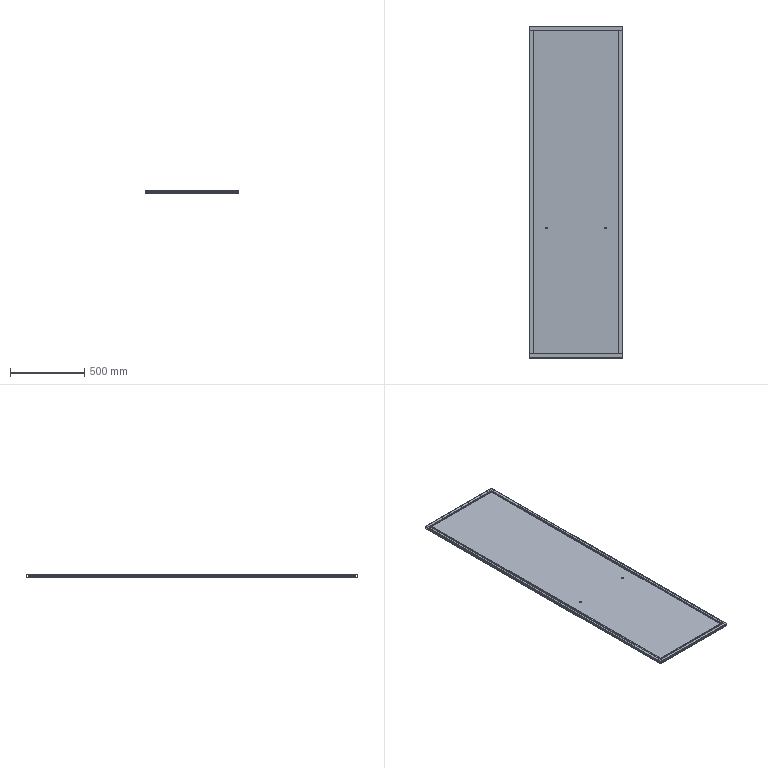Part | SolidWorks | features ICE 2, Cut 1, WeldMemberFeat 1, WeldmentFeature 1 | 5 solids | 171 faces | box 630 x 2236 x 18 mm | volume 13957397 mm3 | plane 98 | cylinder 73 | commonest cylinder face diameters 1.1 x24 3.6 x20 5.8 x20 1 x5 12 x4